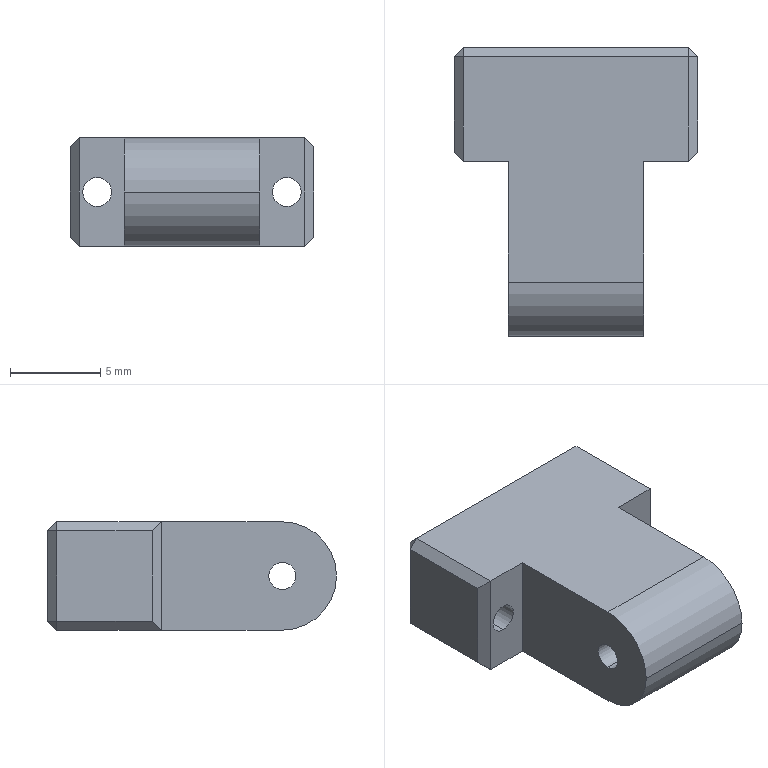Part | SolidWorks | features HoleWzd 2, MirrorPattern 2, Chamfer 1, Extrusion 1, Fillet 1, ICE 1 | 1 solid | 31 faces | box 13.5 x 16 x 6 mm | volume 870.216 mm3 | plane 23 | cylinder 8 | commonest cylinder face diameters 1.6 x4 1.5 x2 6 x2
STEP:
#1=CARTESIAN_POINT('',(9.,-6.3,2.2));
#2=VERTEX_POINT('',#1);
#3=CARTESIAN_POINT('',(9.,-6.3,3.8));
#4=VERTEX_POINT('',#3);
#5=CARTESIAN_POINT('',(9.,-6.3,3.));
#6=DIRECTION('',(0.,1.,0.));
#7=DIRECTION('',(-1.,0.,0.));
#8=AXIS2_PLACEMENT_3D('',#5,#6,#7);
#9=CIRCLE('',#8,0.8);
#10=EDGE_CURVE('',#2,#4,#9,.T.);
#11=ORIENTED_EDGE('',*,*,#10,.F.);
#12=CARTESIAN_POINT('',(9.,0.,2.2));
#13=VERTEX_POINT('',#12);
#14=CARTESIAN_POINT('',(9.,0.,2.2));
#15=DIRECTION('',(0.,1.,0.));
#16=VECTOR('',#15,1000.);
#17=LINE('',#14,#16);
#18=EDGE_CURVE('',#2,#13,#17,.T.);
#19=ORIENTED_EDGE('',*,*,#18,.T.);
#20=CARTESIAN_POINT('',(9.,0.,3.8));
#21=VERTEX_POINT('',#20);
#22=CARTESIAN_POINT('',(9.,0.,3.));
#23=DIRECTION('',(0.,1.,0.));
#24=DIRECTION('',(0.,0.,1.));
#25=AXIS2_PLACEMENT_3D('',#22,#23,#24);
#26=CIRCLE('',#25,0.8);
#27=EDGE_CURVE('',#13,#21,#26,.T.);
#28=ORIENTED_EDGE('',*,*,#27,.T.);
#29=CARTESIAN_POINT('',(9.,0.,3.8));
#30=DIRECTION('',(0.,1.,0.));
#31=VECTOR('',#30,1000.);
#32=LINE('',#29,#31);
#33=EDGE_CURVE('',#4,#21,#32,.T.);
#34=ORIENTED_EDGE('',*,*,#33,.F.);
#35=EDGE_LOOP('',(#11,#19,#28,#34));
#36=FACE_OUTER_BOUND('',#35,.T.);
#37=CARTESIAN_POINT('',(9.,0.,3.));
#38=DIRECTION('',(0.,1.,0.));
#39=DIRECTION('',(0.,0.,1.));
#40=AXIS2_PLACEMENT_3D('',#37,#38,#39);
#41=CYLINDRICAL_SURFACE('',#40,0.8);
#42=ADVANCED_FACE('',(#36),#41,.F.);
#43=CARTESIAN_POINT('',(-1.5,-6.3,3.8));
#44=VERTEX_POINT('',#43);
#45=CARTESIAN_POINT('',(-1.5,-6.3,2.2));
#46=VERTEX_POINT('',#45);
#47=CARTESIAN_POINT('',(-1.5,-6.3,3.));
#48=DIRECTION('',(0.,-1.,0.));
#49=DIRECTION('',(1.,0.,0.));
#50=AXIS2_PLACEMENT_3D('',#47,#48,#49);
#51=CIRCLE('',#50,0.8);
#52=EDGE_CURVE('',#44,#46,#51,.T.);
#53=ORIENTED_EDGE('',*,*,#52,.T.);
#54=CARTESIAN_POINT('',(-1.5,0.,2.2));
#55=VERTEX_POINT('',#54);
#56=CARTESIAN_POINT('',(-1.5,0.,2.2));
#57=DIRECTION('',(0.,1.,0.));
#58=VECTOR('',#57,1000.);
#59=LINE('',#56,#58);
#60=EDGE_CURVE('',#46,#55,#59,.T.);
#61=ORIENTED_EDGE('',*,*,#60,.T.);
#62=CARTESIAN_POINT('',(-1.5,0.,3.8));
#63=VERTEX_POINT('',#62);
#64=CARTESIAN_POINT('',(-1.5,0.,3.));
#65=DIRECTION('',(0.,1.,0.));
#66=DIRECTION('',(0.,0.,1.));
#67=AXIS2_PLACEMENT_3D('',#64,#65,#66);
#68=CIRCLE('',#67,0.8);
#69=EDGE_CURVE('',#55,#63,#68,.T.);
#70=ORIENTED_EDGE('',*,*,#69,.T.);
#71=CARTESIAN_POINT('',(-1.5,0.,3.8));
#72=DIRECTION('',(0.,1.,0.));
#73=VECTOR('',#72,1000.);
#74=LINE('',#71,#73);
#75=EDGE_CURVE('',#44,#63,#74,.T.);
#76=ORIENTED_EDGE('',*,*,#75,.F.);
#77=EDGE_LOOP('',(#53,#61,#70,#76));
#78=FACE_OUTER_BOUND('',#77,.T.);
#79=CARTESIAN_POINT('',(-1.5,0.,3.));
#80=DIRECTION('',(0.,1.,0.));
#81=DIRECTION('',(0.,0.,1.));
#82=AXIS2_PLACEMENT_3D('',#79,#80,#81);
#83=CYLINDRICAL_SURFACE('',#82,0.8);
#84=ADVANCED_FACE('',(#78),#83,.F.);
#85=CARTESIAN_POINT('',(0.,-13.,3.75));
#86=VERTEX_POINT('',#85);
#87=CARTESIAN_POINT('',(0.,-13.,2.25));
#88=VERTEX_POINT('',#87);
#89=CARTESIAN_POINT('',(0.,-13.,3.));
#90=DIRECTION('',(1.,0.,0.));
#91=DIRECTION('',(0.,1.,0.));
#92=AXIS2_PLACEMENT_3D('',#89,#90,#91);
#93=CIRCLE('',#92,0.75);
#94=EDGE_CURVE('',#86,#88,#93,.T.);
#95=ORIENTED_EDGE('',*,*,#94,.F.);
#96=CARTESIAN_POINT('',(7.5,-13.,3.75));
#97=VERTEX_POINT('',#96);
#98=CARTESIAN_POINT('',(7.5,-13.,3.75));
#99=DIRECTION('',(1.,0.,0.));
#100=VECTOR('',#99,1000.);
#101=LINE('',#98,#100);
#102=EDGE_CURVE('',#86,#97,#101,.T.);
#103=ORIENTED_EDGE('',*,*,#102,.T.);
#104=CARTESIAN_POINT('',(7.5,-13.,2.25));
#105=VERTEX_POINT('',#104);
#106=CARTESIAN_POINT('',(7.5,-13.,3.));
#107=DIRECTION('',(1.,0.,0.));
#108=DIRECTION('',(0.,0.,-1.));
#109=AXIS2_PLACEMENT_3D('',#106,#107,#108);
#110=CIRCLE('',#109,0.75);
#111=EDGE_CURVE('',#97,#105,#110,.T.);
#112=ORIENTED_EDGE('',*,*,#111,.T.);
#113=CARTESIAN_POINT('',(7.5,-13.,2.25));
#114=DIRECTION('',(1.,0.,0.));
#115=VECTOR('',#114,1000.);
#116=LINE('',#113,#115);
#117=EDGE_CURVE('',#88,#105,#116,.T.);
#118=ORIENTED_EDGE('',*,*,#117,.F.);
#119=EDGE_LOOP('',(#95,#103,#112,#118));
#120=FACE_OUTER_BOUND('',#119,.T.);
#121=CARTESIAN_POINT('',(7.5,-13.,3.));
#122=DIRECTION('',(1.,0.,0.));
#123=DIRECTION('',(0.,0.,-1.));
#124=AXIS2_PLACEMENT_3D('',#121,#122,#123);
#125=CYLINDRICAL_SURFACE('',#124,0.75);
#126=ADVANCED_FACE('',(#120),#125,.F.);
#127=CARTESIAN_POINT('',(9.,0.,3.));
#128=DIRECTION('',(0.,1.,0.));
#129=DIRECTION('',(0.,0.,1.));
#130=AXIS2_PLACEMENT_3D('',#127,#128,#129);
#131=CIRCLE('',#130,0.8);
#132=EDGE_CURVE('',#21,#13,#131,.T.);
#133=ORIENTED_EDGE('',*,*,#132,.F.);
#134=ORIENTED_EDGE('',*,*,#27,.F.);
#135=EDGE_LOOP('',(#133,#134));
#136=FACE_BOUND('',#135,.T.);
#137=CARTESIAN_POINT('',(-1.5,0.,3.));
#138=DIRECTION('',(0.,1.,0.));
#139=DIRECTION('',(0.,0.,1.));
#140=AXIS2_PLACEMENT_3D('',#137,#138,#139);
#141=CIRCLE('',#140,0.8);
#142=EDGE_CURVE('',#63,#55,#141,.T.);
#143=ORIENTED_EDGE('',*,*,#142,.F.);
#144=ORIENTED_EDGE('',*,*,#69,.F.);
#145=EDGE_LOOP('',(#143,#144));
#146=FACE_BOUND('',#145,.T.);
#147=CARTESIAN_POINT('',(-2.5,0.,5.5));
#148=VERTEX_POINT('',#147);
#149=CARTESIAN_POINT('',(10.,0.,5.5));
#150=VERTEX_POINT('',#149);
#151=CARTESIAN_POINT('',(10.5,0.,5.5));
#152=DIRECTION('',(1.,0.,0.));
#153=VECTOR('',#152,1000.);
#154=LINE('',#151,#153);
#155=EDGE_CURVE('',#148,#150,#154,.T.);
#156=ORIENTED_EDGE('',*,*,#155,.T.);
#157=CARTESIAN_POINT('',(10.,0.,0.5));
#158=VERTEX_POINT('',#157);
#159=CARTESIAN_POINT('',(10.,0.,6.));
#160=DIRECTION('',(0.,0.,-1.));
#161=VECTOR('',#160,1000.);
#162=LINE('',#159,#161);
#163=EDGE_CURVE('',#150,#158,#162,.T.);
#164=ORIENTED_EDGE('',*,*,#163,.T.);
#165=CARTESIAN_POINT('',(-2.5,0.,0.5));
#166=VERTEX_POINT('',#165);
#167=CARTESIAN_POINT('',(0.,0.,0.5));
#168=DIRECTION('',(-1.,0.,0.));
#169=VECTOR('',#168,1000.);
#170=LINE('',#167,#169);
#171=EDGE_CURVE('',#158,#166,#170,.T.);
#172=ORIENTED_EDGE('',*,*,#171,.T.);
#173=CARTESIAN_POINT('',(-2.5,0.,6.));
#174=DIRECTION('',(0.,0.,1.));
#175=VECTOR('',#174,1000.);
#176=LINE('',#173,#175);
#177=EDGE_CURVE('',#166,#148,#176,.T.);
#178=ORIENTED_EDGE('',*,*,#177,.T.);
#179=EDGE_LOOP('',(#156,#164,#172,#178));
#180=FACE_OUTER_BOUND('',#179,.T.);
#181=CARTESIAN_POINT('',(0.,0.,6.));
#182=DIRECTION('',(0.,1.,0.));
#183=DIRECTION('',(0.,0.,1.));
#184=AXIS2_PLACEMENT_3D('',#181,#182,#183);
#185=PLANE('',#184);
#186=ADVANCED_FACE('',(#136,#146,#180),#185,.T.);
#187=CARTESIAN_POINT('',(0.,-13.,3.));
#188=DIRECTION('',(1.,0.,0.));
#189=DIRECTION('',(0.,1.,0.));
#190=AXIS2_PLACEMENT_3D('',#187,#188,#189);
#191=CIRCLE('',#190,0.75);
#192=EDGE_CURVE('',#88,#86,#191,.T.);
#193=ORIENTED_EDGE('',*,*,#192,.T.);
#194=ORIENTED_EDGE('',*,*,#94,.T.);
#195=EDGE_LOOP('',(#193,#194));
#196=FACE_BOUND('',#195,.T.);
#197=CARTESIAN_POINT('',(0.,-6.3,0.));
#198=VERTEX_POINT('',#197);
#199=CARTESIAN_POINT('',(0.,-13.,0.));
#200=VERTEX_POINT('',#199);
#201=CARTESIAN_POINT('',(0.,0.,0.));
#202=DIRECTION('',(0.,-1.,0.));
#203=VECTOR('',#202,1000.);
#204=LINE('',#201,#203);
#205=EDGE_CURVE('',#198,#200,#204,.T.);
#206=ORIENTED_EDGE('',*,*,#205,.T.);
#207=CARTESIAN_POINT('',(0.,-16.,3.));
#208=VERTEX_POINT('',#207);
#209=CARTESIAN_POINT('',(0.,-13.,3.));
#210=DIRECTION('',(-1.,0.,0.));
#211=DIRECTION('',(0.,1.,0.));
#212=AXIS2_PLACEMENT_3D('',#209,#210,#211);
#213=CIRCLE('',#212,3.);
#214=EDGE_CURVE('',#200,#208,#213,.T.);
#215=ORIENTED_EDGE('',*,*,#214,.T.);
#216=CARTESIAN_POINT('',(0.,-13.,6.));
#217=VERTEX_POINT('',#216);
#218=CARTESIAN_POINT('',(0.,-13.,3.));
#219=DIRECTION('',(-1.,0.,0.));
#220=DIRECTION('',(0.,1.,0.));
#221=AXIS2_PLACEMENT_3D('',#218,#219,#220);
#222=CIRCLE('',#221,3.);
#223=EDGE_CURVE('',#208,#217,#222,.T.);
#224=ORIENTED_EDGE('',*,*,#223,.T.);
#225=CARTESIAN_POINT('',(0.,-6.3,6.));
#226=VERTEX_POINT('',#225);
#227=CARTESIAN_POINT('',(0.,0.,6.));
#228=DIRECTION('',(0.,-1.,0.));
#229=VECTOR('',#228,1000.);
#230=LINE('',#227,#229);
#231=EDGE_CURVE('',#226,#217,#230,.T.);
#232=ORIENTED_EDGE('',*,*,#231,.F.);
#233=CARTESIAN_POINT('',(0.,-6.3,6.));
#234=DIRECTION('',(0.,0.,-1.));
#235=VECTOR('',#234,1000.);
#236=LINE('',#233,#235);
#237=EDGE_CURVE('',#226,#198,#236,.T.);
#238=ORIENTED_EDGE('',*,*,#237,.T.);
#239=EDGE_LOOP('',(#206,#215,#224,#232,#238));
#240=FACE_OUTER_BOUND('',#239,.T.);
#241=CARTESIAN_POINT('',(0.,0.,6.));
#242=DIRECTION('',(1.,0.,0.));
#243=DIRECTION('',(0.,1.,0.));
#244=AXIS2_PLACEMENT_3D('',#241,#242,#243);
#245=PLANE('',#244);
#246=ADVANCED_FACE('',(#196,#240),#245,.F.);
#247=CARTESIAN_POINT('',(7.5,-13.,3.));
#248=DIRECTION('',(1.,0.,0.));
#249=DIRECTION('',(0.,0.,-1.));
#250=AXIS2_PLACEMENT_3D('',#247,#248,#249);
#251=CIRCLE('',#250,0.75);
#252=EDGE_CURVE('',#105,#97,#251,.T.);
#253=ORIENTED_EDGE('',*,*,#252,.F.);
#254=ORIENTED_EDGE('',*,*,#111,.F.);
#255=EDGE_LOOP('',(#253,#254));
#256=FACE_BOUND('',#255,.T.);
#257=CARTESIAN_POINT('',(7.5,-13.,6.));
#258=VERTEX_POINT('',#257);
#259=CARTESIAN_POINT('',(7.5,-16.,3.));
#260=VERTEX_POINT('',#259);
#261=CARTESIAN_POINT('',(7.5,-13.,3.));
#262=DIRECTION('',(1.,0.,0.));
#263=DIRECTION('',(0.,1.,0.));
#264=AXIS2_PLACEMENT_3D('',#261,#262,#263);
#265=CIRCLE('',#264,3.);
#266=EDGE_CURVE('',#258,#260,#265,.T.);
#267=ORIENTED_EDGE('',*,*,#266,.T.);
#268=CARTESIAN_POINT('',(7.5,-13.,0.));
#269=VERTEX_POINT('',#268);
#270=CARTESIAN_POINT('',(7.5,-13.,3.));
#271=DIRECTION('',(1.,0.,0.));
#272=DIRECTION('',(0.,1.,0.));
#273=AXIS2_PLACEMENT_3D('',#270,#271,#272);
#274=CIRCLE('',#273,3.);
#275=EDGE_CURVE('',#260,#269,#274,.T.);
#276=ORIENTED_EDGE('',*,*,#275,.T.);
#277=CARTESIAN_POINT('',(7.5,-6.3,0.));
#278=VERTEX_POINT('',#277);
#279=CARTESIAN_POINT('',(7.5,0.,0.));
#280=DIRECTION('',(0.,-1.,0.));
#281=VECTOR('',#280,1000.);
#282=LINE('',#279,#281);
#283=EDGE_CURVE('',#278,#269,#282,.T.);
#284=ORIENTED_EDGE('',*,*,#283,.F.);
#285=CARTESIAN_POINT('',(7.5,-6.3,6.));
#286=VERTEX_POINT('',#285);
#287=CARTESIAN_POINT('',(7.5,-6.3,6.));
#288=DIRECTION('',(0.,0.,-1.));
#289=VECTOR('',#288,1000.);
#290=LINE('',#287,#289);
#291=EDGE_CURVE('',#286,#278,#290,.T.);
#292=ORIENTED_EDGE('',*,*,#291,.F.);
#293=CARTESIAN_POINT('',(7.5,0.,6.));
#294=DIRECTION('',(0.,-1.,0.));
#295=VECTOR('',#294,1000.);
#296=LINE('',#293,#295);
#297=EDGE_CURVE('',#286,#258,#296,.T.);
#298=ORIENTED_EDGE('',*,*,#297,.T.);
#299=EDGE_LOOP('',(#267,#276,#284,#292,#298));
#300=FACE_OUTER_BOUND('',#299,.T.);
#301=CARTESIAN_POINT('',(7.5,0.,6.));
#302=DIRECTION('',(1.,0.,0.));
#303=DIRECTION('',(0.,1.,0.));
#304=AXIS2_PLACEMENT_3D('',#301,#302,#303);
#305=PLANE('',#304);
#306=ADVANCED_FACE('',(#256,#300),#305,.T.);
#307=CARTESIAN_POINT('',(10.,-0.5,6.));
#308=VERTEX_POINT('',#307);
#309=CARTESIAN_POINT('',(-2.5,-0.5,6.));
#310=VERTEX_POINT('',#309);
#311=CARTESIAN_POINT('',(-3.,-0.5,6.));
#312=DIRECTION('',(-1.,0.,0.));
#313=VECTOR('',#312,1000.);
#314=LINE('',#311,#313);
#315=EDGE_CURVE('',#308,#310,#314,.T.);
#316=ORIENTED_EDGE('',*,*,#315,.T.);
#317=CARTESIAN_POINT('',(-2.5,-6.3,6.));
#318=VERTEX_POINT('',#317);
#319=CARTESIAN_POINT('',(-2.5,-6.3,6.));
#320=DIRECTION('',(0.,-1.,0.));
#321=VECTOR('',#320,1000.);
#322=LINE('',#319,#321);
#323=EDGE_CURVE('',#310,#318,#322,.T.);
#324=ORIENTED_EDGE('',*,*,#323,.T.);
#325=CARTESIAN_POINT('',(-3.,-6.3,6.));
#326=DIRECTION('',(1.,0.,0.));
#327=VECTOR('',#326,1000.);
#328=LINE('',#325,#327);
#329=EDGE_CURVE('',#318,#226,#328,.T.);
#330=ORIENTED_EDGE('',*,*,#329,.T.);
#331=ORIENTED_EDGE('',*,*,#231,.T.);
#332=CARTESIAN_POINT('',(0.,-13.,6.));
#333=DIRECTION('',(1.,0.,0.));
#334=VECTOR('',#333,1000.);
#335=LINE('',#332,#334);
#336=EDGE_CURVE('',#217,#258,#335,.T.);
#337=ORIENTED_EDGE('',*,*,#336,.T.);
#338=ORIENTED_EDGE('',*,*,#297,.F.);
#339=CARTESIAN_POINT('',(10.,-6.3,6.));
#340=VERTEX_POINT('',#339);
#341=CARTESIAN_POINT('',(10.5,-6.3,6.));
#342=DIRECTION('',(-1.,0.,0.));
#343=VECTOR('',#342,1000.);
#344=LINE('',#341,#343);
#345=EDGE_CURVE('',#340,#286,#344,.T.);
#346=ORIENTED_EDGE('',*,*,#345,.F.);
#347=CARTESIAN_POINT('',(10.,0.,6.));
#348=DIRECTION('',(0.,1.,0.));
#349=VECTOR('',#348,1000.);
#350=LINE('',#347,#349);
#351=EDGE_CURVE('',#340,#308,#350,.T.);
#352=ORIENTED_EDGE('',*,*,#351,.T.);
#353=EDGE_LOOP('',(#316,#324,#330,#331,#337,#338,#346,#352));
#354=FACE_OUTER_BOUND('',#353,.T.);
#355=CARTESIAN_POINT('',(0.,0.,6.));
#356=DIRECTION('',(0.,0.,-1.));
#357=DIRECTION('',(-1.,0.,0.));
#358=AXIS2_PLACEMENT_3D('',#355,#356,#357);
#359=PLANE('',#358);
#360=ADVANCED_FACE('',(#354),#359,.F.);
#361=CARTESIAN_POINT('',(-2.5,-6.3,0.));
#362=VERTEX_POINT('',#361);
#363=CARTESIAN_POINT('',(-3.,-6.3,0.));
#364=DIRECTION('',(1.,0.,0.));
#365=VECTOR('',#364,1000.);
#366=LINE('',#363,#365);
#367=EDGE_CURVE('',#362,#198,#366,.T.);
#368=ORIENTED_EDGE('',*,*,#367,.F.);
#369=CARTESIAN_POINT('',(-2.5,-0.5,0.));
#370=VERTEX_POINT('',#369);
#371=CARTESIAN_POINT('',(-2.5,0.,0.));
#372=DIRECTION('',(0.,1.,0.));
#373=VECTOR('',#372,1000.);
#374=LINE('',#371,#373);
#375=EDGE_CURVE('',#362,#370,#374,.T.);
#376=ORIENTED_EDGE('',*,*,#375,.T.);
#377=CARTESIAN_POINT('',(10.,-0.5,0.));
#378=VERTEX_POINT('',#377);
#379=CARTESIAN_POINT('',(0.,-0.5,0.));
#380=DIRECTION('',(1.,0.,0.));
#381=VECTOR('',#380,1000.);
#382=LINE('',#379,#381);
#383=EDGE_CURVE('',#370,#378,#382,.T.);
#384=ORIENTED_EDGE('',*,*,#383,.T.);
#385=CARTESIAN_POINT('',(10.,-6.3,0.));
#386=VERTEX_POINT('',#385);
#387=CARTESIAN_POINT('',(10.,0.,0.));
#388=DIRECTION('',(0.,-1.,0.));
#389=VECTOR('',#388,1000.);
#390=LINE('',#387,#389);
#391=EDGE_CURVE('',#378,#386,#390,.T.);
#392=ORIENTED_EDGE('',*,*,#391,.T.);
#393=CARTESIAN_POINT('',(10.5,-6.3,0.));
#394=DIRECTION('',(-1.,0.,0.));
#395=VECTOR('',#394,1000.);
#396=LINE('',#393,#395);
#397=EDGE_CURVE('',#386,#278,#396,.T.);
#398=ORIENTED_EDGE('',*,*,#397,.T.);
#399=ORIENTED_EDGE('',*,*,#283,.T.);
#400=CARTESIAN_POINT('',(0.,-13.,0.));
#401=DIRECTION('',(-1.,0.,0.));
#402=VECTOR('',#401,1000.);
#403=LINE('',#400,#402);
#404=EDGE_CURVE('',#269,#200,#403,.T.);
#405=ORIENTED_EDGE('',*,*,#404,.T.);
#406=ORIENTED_EDGE('',*,*,#205,.F.);
#407=EDGE_LOOP('',(#368,#376,#384,#392,#398,#399,#405,#406));
#408=FACE_OUTER_BOUND('',#407,.T.);
#409=CARTESIAN_POINT('',(0.,0.,0.));
#410=DIRECTION('',(0.,0.,-1.));
#411=DIRECTION('',(-1.,0.,0.));
#412=AXIS2_PLACEMENT_3D('',#409,#410,#411);
#413=PLANE('',#412);
#414=ADVANCED_FACE('',(#408),#413,.T.);
#415=CARTESIAN_POINT('',(9.,-6.3,3.));
#416=DIRECTION('',(0.,1.,0.));
#417=DIRECTION('',(-1.,0.,0.));
#418=AXIS2_PLACEMENT_3D('',#415,#416,#417);
#419=CIRCLE('',#418,0.8);
#420=EDGE_CURVE('',#4,#2,#419,.T.);
#421=ORIENTED_EDGE('',*,*,#420,.T.);
#422=ORIENTED_EDGE('',*,*,#10,.T.);
#423=EDGE_LOOP('',(#421,#422));
#424=FACE_BOUND('',#423,.T.);
#425=ORIENTED_EDGE('',*,*,#397,.F.);
#426=CARTESIAN_POINT('',(10.,-6.3,6.));
#427=DIRECTION('',(0.,0.,1.));
#428=VECTOR('',#427,1000.);
#429=LINE('',#426,#428);
#430=EDGE_CURVE('',#386,#340,#429,.T.);
#431=ORIENTED_EDGE('',*,*,#430,.T.);
#432=ORIENTED_EDGE('',*,*,#345,.T.);
#433=ORIENTED_EDGE('',*,*,#291,.T.);
#434=EDGE_LOOP('',(#425,#431,#432,#433));
#435=FACE_OUTER_BOUND('',#434,.T.);
#436=CARTESIAN_POINT('',(10.5,-6.3,6.));
#437=DIRECTION('',(0.,1.,0.));
#438=DIRECTION('',(-1.,0.,0.));
#439=AXIS2_PLACEMENT_3D('',#436,#437,#438);
#440=PLANE('',#439);
#441=ADVANCED_FACE('',(#424,#435),#440,.F.);
#442=CARTESIAN_POINT('',(10.5,-5.8,5.5));
#443=VERTEX_POINT('',#442);
#444=CARTESIAN_POINT('',(10.5,-5.8,0.5));
#445=VERTEX_POINT('',#444);
#446=CARTESIAN_POINT('',(10.5,-5.8,0.));
#447=DIRECTION('',(0.,0.,-1.));
#448=VECTOR('',#447,1000.);
#449=LINE('',#446,#448);
#450=EDGE_CURVE('',#443,#445,#449,.T.);
#451=ORIENTED_EDGE('',*,*,#450,.T.);
#452=CARTESIAN_POINT('',(10.5,-0.5,0.5));
#453=VERTEX_POINT('',#452);
#454=CARTESIAN_POINT('',(10.5,0.,0.5));
#455=DIRECTION('',(0.,1.,0.));
#456=VECTOR('',#455,1000.);
#457=LINE('',#454,#456);
#458=EDGE_CURVE('',#445,#453,#457,.T.);
#459=ORIENTED_EDGE('',*,*,#458,.T.);
#460=CARTESIAN_POINT('',(10.5,-0.5,5.5));
#461=VERTEX_POINT('',#460);
#462=CARTESIAN_POINT('',(10.5,-0.5,0.));
#463=DIRECTION('',(0.,0.,1.));
#464=VECTOR('',#463,1000.);
#465=LINE('',#462,#464);
#466=EDGE_CURVE('',#453,#461,#465,.T.);
#467=ORIENTED_EDGE('',*,*,#466,.T.);
#468=CARTESIAN_POINT('',(10.5,-6.3,5.5));
#469=DIRECTION('',(0.,-1.,0.));
#470=VECTOR('',#469,1000.);
#471=LINE('',#468,#470);
#472=EDGE_CURVE('',#461,#443,#471,.T.);
#473=ORIENTED_EDGE('',*,*,#472,.T.);
#474=EDGE_LOOP('',(#451,#459,#467,#473));
#475=FACE_OUTER_BOUND('',#474,.T.);
#476=CARTESIAN_POINT('',(10.5,0.,0.));
#477=DIRECTION('',(1.,0.,0.));
#478=DIRECTION('',(0.,1.,0.));
#479=AXIS2_PLACEMENT_3D('',#476,#477,#478);
#480=PLANE('',#479);
#481=ADVANCED_FACE('',(#475),#480,.T.);
#482=ORIENTED_EDGE('',*,*,#52,.F.);
#483=CARTESIAN_POINT('',(-1.5,-6.3,3.));
#484=DIRECTION('',(0.,-1.,0.));
#485=DIRECTION('',(1.,0.,0.));
#486=AXIS2_PLACEMENT_3D('',#483,#484,#485);
#487=CIRCLE('',#486,0.8);
#488=EDGE_CURVE('',#46,#44,#487,.T.);
#489=ORIENTED_EDGE('',*,*,#488,.F.);
#490=EDGE_LOOP('',(#482,#489));
#491=FACE_BOUND('',#490,.T.);
#492=ORIENTED_EDGE('',*,*,#329,.F.);
#493=CARTESIAN_POINT('',(-2.5,-6.3,6.));
#494=DIRECTION('',(0.,0.,-1.));
#495=VECTOR('',#494,1000.);
#496=LINE('',#493,#495);
#497=EDGE_CURVE('',#318,#362,#496,.T.);
#498=ORIENTED_EDGE('',*,*,#497,.T.);
#499=ORIENTED_EDGE('',*,*,#367,.T.);
#500=ORIENTED_EDGE('',*,*,#237,.F.);
#501=EDGE_LOOP('',(#492,#498,#499,#500));
#502=FACE_OUTER_BOUND('',#501,.T.);
#503=CARTESIAN_POINT('',(-3.,-6.3,6.));
#504=DIRECTION('',(0.,-1.,0.));
#505=DIRECTION('',(1.,0.,0.));
#506=AXIS2_PLACEMENT_3D('',#503,#504,#505);
#507=PLANE('',#506);
#508=ADVANCED_FACE('',(#491,#502),#507,.T.);
#509=CARTESIAN_POINT('',(-3.,-0.5,0.5));
#510=VERTEX_POINT('',#509);
#511=CARTESIAN_POINT('',(-3.,-5.8,0.5));
#512=VERTEX_POINT('',#511);
#513=CARTESIAN_POINT('',(-3.,0.,0.5));
#514=DIRECTION('',(0.,-1.,0.));
#515=VECTOR('',#514,1000.);
#516=LINE('',#513,#515);
#517=EDGE_CURVE('',#510,#512,#516,.T.);
#518=ORIENTED_EDGE('',*,*,#517,.T.);
#519=CARTESIAN_POINT('',(-3.,-5.8,5.5));
#520=VERTEX_POINT('',#519);
#521=CARTESIAN_POINT('',(-3.,-5.8,0.));
#522=DIRECTION('',(0.,0.,1.));
#523=VECTOR('',#522,1000.);
#524=LINE('',#521,#523);
#525=EDGE_CURVE('',#512,#520,#524,.T.);
#526=ORIENTED_EDGE('',*,*,#525,.T.);
#527=CARTESIAN_POINT('',(-3.,-0.5,5.5));
#528=VERTEX_POINT('',#527);
#529=CARTESIAN_POINT('',(-3.,0.,5.5));
#530=DIRECTION('',(0.,1.,0.));
#531=VECTOR('',#530,1000.);
#532=LINE('',#529,#531);
#533=EDGE_CURVE('',#520,#528,#532,.T.);
#534=ORIENTED_EDGE('',*,*,#533,.T.);
#535=CARTESIAN_POINT('',(-3.,-0.5,0.));
#536=DIRECTION('',(0.,0.,-1.));
#537=VECTOR('',#536,1000.);
#538=LINE('',#535,#537);
#539=EDGE_CURVE('',#528,#510,#538,.T.);
#540=ORIENTED_EDGE('',*,*,#539,.T.);
#541=EDGE_LOOP('',(#518,#526,#534,#540));
#542=FACE_OUTER_BOUND('',#541,.T.);
#543=CARTESIAN_POINT('',(-3.,0.,0.));
#544=DIRECTION('',(-1.,0.,0.));
#545=DIRECTION('',(0.,1.,0.));
#546=AXIS2_PLACEMENT_3D('',#543,#544,#545);
#547=PLANE('',#546);
#548=ADVANCED_FACE('',(#542),#547,.T.);
#549=ORIENTED_EDGE('',*,*,#102,.F.);
#550=ORIENTED_EDGE('',*,*,#192,.F.);
#551=ORIENTED_EDGE('',*,*,#117,.T.);
#552=ORIENTED_EDGE('',*,*,#252,.T.);
#553=EDGE_LOOP('',(#549,#550,#551,#552));
#554=FACE_OUTER_BOUND('',#553,.T.);
#555=CARTESIAN_POINT('',(7.5,-13.,3.));
#556=DIRECTION('',(1.,0.,0.));
#557=DIRECTION('',(0.,0.,-1.));
#558=AXIS2_PLACEMENT_3D('',#555,#556,#557);
#559=CYLINDRICAL_SURFACE('',#558,0.75);
#560=ADVANCED_FACE('',(#554),#559,.F.);
#561=ORIENTED_EDGE('',*,*,#336,.F.);
#562=ORIENTED_EDGE('',*,*,#223,.F.);
#563=CARTESIAN_POINT('',(0.,-16.,3.));
#564=DIRECTION('',(-1.,0.,0.));
#565=VECTOR('',#564,1000.);
#566=LINE('',#563,#565);
#567=EDGE_CURVE('',#260,#208,#566,.T.);
#568=ORIENTED_EDGE('',*,*,#567,.F.);
#569=ORIENTED_EDGE('',*,*,#266,.F.);
#570=EDGE_LOOP('',(#561,#562,#568,#569));
#571=FACE_OUTER_BOUND('',#570,.T.);
#572=CARTESIAN_POINT('',(0.,-13.,3.));
#573=DIRECTION('',(1.,0.,0.));
#574=DIRECTION('',(0.,0.,-1.));
#575=AXIS2_PLACEMENT_3D('',#572,#573,#574);
#576=CYLINDRICAL_SURFACE('',#575,3.);
#577=ADVANCED_FACE('',(#571),#576,.T.);
#578=ORIENTED_EDGE('',*,*,#214,.F.);
#579=ORIENTED_EDGE('',*,*,#404,.F.);
#580=ORIENTED_EDGE('',*,*,#275,.F.);
#581=ORIENTED_EDGE('',*,*,#567,.T.);
#582=EDGE_LOOP('',(#578,#579,#580,#581));
#583=FACE_OUTER_BOUND('',#582,.T.);
#584=CARTESIAN_POINT('',(0.,-13.,3.));
#585=DIRECTION('',(-1.,0.,0.));
#586=DIRECTION('',(0.,0.,1.));
#587=AXIS2_PLACEMENT_3D('',#584,#585,#586);
#588=CYLINDRICAL_SURFACE('',#587,3.);
#589=ADVANCED_FACE('',(#583),#588,.T.);
#590=CARTESIAN_POINT('',(10.333,-5.967,0.3333));
#591=DIRECTION('',(-0.5774,-0.5774,-0.5774));
#592=VECTOR('',#591,1000.);
#593=LINE('',#590,#592);
#594=EDGE_CURVE('',#445,#386,#593,.T.);
#595=ORIENTED_EDGE('',*,*,#594,.F.);
#596=ORIENTED_EDGE('',*,*,#450,.F.);
#597=CARTESIAN_POINT('',(12.433,-3.867,3.567));
#598=DIRECTION('',(0.5774,0.5774,-0.5774));
#599=VECTOR('',#598,1000.);
#600=LINE('',#597,#599);
#601=EDGE_CURVE('',#340,#443,#600,.T.);
#602=ORIENTED_EDGE('',*,*,#601,.F.);
#603=ORIENTED_EDGE('',*,*,#430,.F.);
#604=EDGE_LOOP('',(#595,#596,#602,#603));
#605=FACE_OUTER_BOUND('',#604,.T.);
#606=CARTESIAN_POINT('',(10.5,-5.8,0.));
#607=DIRECTION('',(0.7071,-0.7071,0.));
#608=DIRECTION('',(0.,0.,1.));
#609=AXIS2_PLACEMENT_3D('',#606,#607,#608);
#610=PLANE('',#609);
#611=ADVANCED_FACE('',(#605),#610,.T.);
#612=ORIENTED_EDGE('',*,*,#601,.T.);
#613=ORIENTED_EDGE('',*,*,#472,.F.);
#614=CARTESIAN_POINT('',(10.,-0.5,6.));
#615=DIRECTION('',(0.7071,0.,-0.7071));
#616=VECTOR('',#615,1000.);
#617=LINE('',#614,#616);
#618=EDGE_CURVE('',#308,#461,#617,.T.);
#619=ORIENTED_EDGE('',*,*,#618,.F.);
#620=ORIENTED_EDGE('',*,*,#351,.F.);
#621=EDGE_LOOP('',(#612,#613,#619,#620));
#622=FACE_OUTER_BOUND('',#621,.T.);
#623=CARTESIAN_POINT('',(10.5,0.,5.5));
#624=DIRECTION('',(0.7071,0.,0.7071));
#625=DIRECTION('',(0.,1.,0.));
#626=AXIS2_PLACEMENT_3D('',#623,#624,#625);
#627=PLANE('',#626);
#628=ADVANCED_FACE('',(#622),#627,.T.);
#629=ORIENTED_EDGE('',*,*,#594,.T.);
#630=ORIENTED_EDGE('',*,*,#391,.F.);
#631=CARTESIAN_POINT('',(10.5,-0.5,0.5));
#632=DIRECTION('',(-0.7071,0.,-0.7071));
#633=VECTOR('',#632,1000.);
#634=LINE('',#631,#633);
#635=EDGE_CURVE('',#453,#378,#634,.T.);
#636=ORIENTED_EDGE('',*,*,#635,.F.);
#637=ORIENTED_EDGE('',*,*,#458,.F.);
#638=EDGE_LOOP('',(#629,#630,#636,#637));
#639=FACE_OUTER_BOUND('',#638,.T.);
#640=CARTESIAN_POINT('',(10.5,0.,0.5));
#641=DIRECTION('',(-0.7071,0.,0.7071));
#642=DIRECTION('',(0.,1.,0.));
#643=AXIS2_PLACEMENT_3D('',#640,#641,#642);
#644=PLANE('',#643);
#645=ADVANCED_FACE('',(#639),#644,.F.);
#646=CARTESIAN_POINT('',(10.25,-0.25,5.5));
#647=DIRECTION('',(-0.7071,0.7071,0.));
#648=VECTOR('',#647,1000.);
#649=LINE('',#646,#648);
#650=EDGE_CURVE('',#461,#150,#649,.T.);
#651=ORIENTED_EDGE('',*,*,#650,.F.);
#652=ORIENTED_EDGE('',*,*,#466,.F.);
#653=CARTESIAN_POINT('',(10.5,-0.5,0.5));
#654=DIRECTION('',(0.7071,-0.7071,0.));
#655=VECTOR('',#654,1000.);
#656=LINE('',#653,#655);
#657=EDGE_CURVE('',#158,#453,#656,.T.);
#658=ORIENTED_EDGE('',*,*,#657,.F.);
#659=ORIENTED_EDGE('',*,*,#163,.F.);
#660=EDGE_LOOP('',(#651,#652,#658,#659));
#661=FACE_OUTER_BOUND('',#660,.T.);
#662=CARTESIAN_POINT('',(10.5,-0.5,0.));
#663=DIRECTION('',(-0.7071,-0.7071,0.));
#664=DIRECTION('',(0.,0.,1.));
#665=AXIS2_PLACEMENT_3D('',#662,#663,#664);
#666=PLANE('',#665);
#667=ADVANCED_FACE('',(#661),#666,.F.);
#668=ORIENTED_EDGE('',*,*,#618,.T.);
#669=ORIENTED_EDGE('',*,*,#650,.T.);
#670=CARTESIAN_POINT('',(10.,-0.5,6.));
#671=DIRECTION('',(0.,0.7071,-0.7071));
#672=VECTOR('',#671,1000.);
#673=LINE('',#670,#672);
#674=EDGE_CURVE('',#308,#150,#673,.T.);
#675=ORIENTED_EDGE('',*,*,#674,.F.);
#676=EDGE_LOOP('',(#668,#669,#675));
#677=FACE_OUTER_BOUND('',#676,.T.);
#678=CARTESIAN_POINT('',(10.,-0.5,6.));
#679=DIRECTION('',(0.5774,0.5774,0.5774));
#680=DIRECTION('',(0.,-0.7071,0.7071));
#681=AXIS2_PLACEMENT_3D('',#678,#679,#680);
#682=PLANE('',#681);
#683=ADVANCED_FACE('',(#677),#682,.T.);
#684=ORIENTED_EDGE('',*,*,#657,.T.);
#685=ORIENTED_EDGE('',*,*,#635,.T.);
#686=CARTESIAN_POINT('',(10.,-0.25,0.25));
#687=DIRECTION('',(0.,-0.7071,-0.7071));
#688=VECTOR('',#687,1000.);
#689=LINE('',#686,#688);
#690=EDGE_CURVE('',#158,#378,#689,.T.);
#691=ORIENTED_EDGE('',*,*,#690,.F.);
#692=EDGE_LOOP('',(#684,#685,#691));
#693=FACE_OUTER_BOUND('',#692,.T.);
#694=CARTESIAN_POINT('',(10.5,-0.5,0.5));
#695=DIRECTION('',(0.5774,0.5774,-0.5774));
#696=DIRECTION('',(-0.7071,0.7071,0.));
#697=AXIS2_PLACEMENT_3D('',#694,#695,#696);
#698=PLANE('',#697);
#699=ADVANCED_FACE('',(#693),#698,.T.);
#700=ORIENTED_EDGE('',*,*,#674,.T.);
#701=ORIENTED_EDGE('',*,*,#155,.F.);
#702=CARTESIAN_POINT('',(-2.5,-0.25,5.75));
#703=DIRECTION('',(0.,0.7071,-0.7071));
#704=VECTOR('',#703,1000.);
#705=LINE('',#702,#704);
#706=EDGE_CURVE('',#310,#148,#705,.T.);
#707=ORIENTED_EDGE('',*,*,#706,.F.);
#708=ORIENTED_EDGE('',*,*,#315,.F.);
#709=EDGE_LOOP('',(#700,#701,#707,#708));
#710=FACE_OUTER_BOUND('',#709,.T.);
#711=CARTESIAN_POINT('',(0.,0.,5.5));
#712=DIRECTION('',(0.,0.7071,0.7071));
#713=DIRECTION('',(-1.,0.,0.));
#714=AXIS2_PLACEMENT_3D('',#711,#712,#713);
#715=PLANE('',#714);
#716=ADVANCED_FACE('',(#710),#715,.T.);
#717=ORIENTED_EDGE('',*,*,#690,.T.);
#718=ORIENTED_EDGE('',*,*,#383,.F.);
#719=CARTESIAN_POINT('',(-2.5,-0.5,0.));
#720=DIRECTION('',(0.,-0.7071,-0.7071));
#721=VECTOR('',#720,1000.);
#722=LINE('',#719,#721);
#723=EDGE_CURVE('',#166,#370,#722,.T.);
#724=ORIENTED_EDGE('',*,*,#723,.F.);
#725=ORIENTED_EDGE('',*,*,#171,.F.);
#726=EDGE_LOOP('',(#717,#718,#724,#725));
#727=FACE_OUTER_BOUND('',#726,.T.);
#728=CARTESIAN_POINT('',(0.,-0.5,0.));
#729=DIRECTION('',(0.,-0.7071,0.7071));
#730=DIRECTION('',(1.,0.,0.));
#731=AXIS2_PLACEMENT_3D('',#728,#729,#730);
#732=PLANE('',#731);
#733=ADVANCED_FACE('',(#727),#732,.F.);
#734=CARTESIAN_POINT('',(-3.,-0.5,5.5));
#735=DIRECTION('',(-0.7071,-0.7071,0.));
#736=VECTOR('',#735,1000.);
#737=LINE('',#734,#736);
#738=EDGE_CURVE('',#148,#528,#737,.T.);
#739=ORIENTED_EDGE('',*,*,#738,.F.);
#740=ORIENTED_EDGE('',*,*,#177,.F.);
#741=CARTESIAN_POINT('',(-2.75,-0.25,0.5));
#742=DIRECTION('',(0.7071,0.7071,0.));
#743=VECTOR('',#742,1000.);
#744=LINE('',#741,#743);
#745=EDGE_CURVE('',#510,#166,#744,.T.);
#746=ORIENTED_EDGE('',*,*,#745,.F.);
#747=ORIENTED_EDGE('',*,*,#539,.F.);
#748=EDGE_LOOP('',(#739,#740,#746,#747));
#749=FACE_OUTER_BOUND('',#748,.T.);
#750=CARTESIAN_POINT('',(-2.5,0.,6.));
#751=DIRECTION('',(0.7071,-0.7071,0.));
#752=DIRECTION('',(0.,0.,1.));
#753=AXIS2_PLACEMENT_3D('',#750,#751,#752);
#754=PLANE('',#753);
#755=ADVANCED_FACE('',(#749),#754,.F.);
#756=ORIENTED_EDGE('',*,*,#706,.T.);
#757=ORIENTED_EDGE('',*,*,#738,.T.);
#758=CARTESIAN_POINT('',(-3.,-0.5,5.5));
#759=DIRECTION('',(-0.7071,0.,-0.7071));
#760=VECTOR('',#759,1000.);
#761=LINE('',#758,#760);
#762=EDGE_CURVE('',#310,#528,#761,.T.);
#763=ORIENTED_EDGE('',*,*,#762,.F.);
#764=EDGE_LOOP('',(#756,#757,#763));
#765=FACE_OUTER_BOUND('',#764,.T.);
#766=CARTESIAN_POINT('',(-3.,-0.5,5.5));
#767=DIRECTION('',(-0.5774,0.5774,0.5774));
#768=DIRECTION('',(-0.7071,-0.7071,0.));
#769=AXIS2_PLACEMENT_3D('',#766,#767,#768);
#770=PLANE('',#769);
#771=ADVANCED_FACE('',(#765),#770,.T.);
#772=ORIENTED_EDGE('',*,*,#745,.T.);
#773=ORIENTED_EDGE('',*,*,#723,.T.);
#774=CARTESIAN_POINT('',(-2.5,-0.5,0.));
#775=DIRECTION('',(0.7071,0.,-0.7071));
#776=VECTOR('',#775,1000.);
#777=LINE('',#774,#776);
#778=EDGE_CURVE('',#510,#370,#777,.T.);
#779=ORIENTED_EDGE('',*,*,#778,.F.);
#780=EDGE_LOOP('',(#772,#773,#779));
#781=FACE_OUTER_BOUND('',#780,.T.);
#782=CARTESIAN_POINT('',(-2.5,-0.5,0.));
#783=DIRECTION('',(-0.5774,0.5774,-0.5774));
#784=DIRECTION('',(-0.7071,-0.7071,0.));
#785=AXIS2_PLACEMENT_3D('',#782,#783,#784);
#786=PLANE('',#785);
#787=ADVANCED_FACE('',(#781),#786,.T.);
#788=ORIENTED_EDGE('',*,*,#762,.T.);
#789=ORIENTED_EDGE('',*,*,#533,.F.);
#790=CARTESIAN_POINT('',(-4.6,-4.2,3.9));
#791=DIRECTION('',(-0.5774,0.5774,-0.5774));
#792=VECTOR('',#791,1000.);
#793=LINE('',#790,#792);
#794=EDGE_CURVE('',#318,#520,#793,.T.);
#795=ORIENTED_EDGE('',*,*,#794,.F.);
#796=ORIENTED_EDGE('',*,*,#323,.F.);
#797=EDGE_LOOP('',(#788,#789,#795,#796));
#798=FACE_OUTER_BOUND('',#797,.T.);
#799=CARTESIAN_POINT('',(-2.5,0.,6.));
#800=DIRECTION('',(-0.7071,0.,0.7071));
#801=DIRECTION('',(0.,1.,0.));
#802=AXIS2_PLACEMENT_3D('',#799,#800,#801);
#803=PLANE('',#802);
#804=ADVANCED_FACE('',(#798),#803,.T.);
#805=ORIENTED_EDGE('',*,*,#778,.T.);
#806=ORIENTED_EDGE('',*,*,#375,.F.);
#807=CARTESIAN_POINT('',(-4.6,-4.2,2.1));
#808=DIRECTION('',(0.5774,-0.5774,-0.5774));
#809=VECTOR('',#808,1000.);
#810=LINE('',#807,#809);
#811=EDGE_CURVE('',#512,#362,#810,.T.);
#812=ORIENTED_EDGE('',*,*,#811,.F.);
#813=ORIENTED_EDGE('',*,*,#517,.F.);
#814=EDGE_LOOP('',(#805,#806,#812,#813));
#815=FACE_OUTER_BOUND('',#814,.T.);
#816=CARTESIAN_POINT('',(-2.5,0.,0.));
#817=DIRECTION('',(0.7071,0.,0.7071));
#818=DIRECTION('',(0.,1.,0.));
#819=AXIS2_PLACEMENT_3D('',#816,#817,#818);
#820=PLANE('',#819);
#821=ADVANCED_FACE('',(#815),#820,.F.);
#822=ORIENTED_EDGE('',*,*,#794,.T.);
#823=ORIENTED_EDGE('',*,*,#525,.F.);
#824=ORIENTED_EDGE('',*,*,#811,.T.);
#825=ORIENTED_EDGE('',*,*,#497,.F.);
#826=EDGE_LOOP('',(#822,#823,#824,#825));
#827=FACE_OUTER_BOUND('',#826,.T.);
#828=CARTESIAN_POINT('',(-2.5,-6.3,6.));
#829=DIRECTION('',(0.7071,0.7071,0.));
#830=DIRECTION('',(0.,0.,-1.));
#831=AXIS2_PLACEMENT_3D('',#828,#829,#830);
#832=PLANE('',#831);
#833=ADVANCED_FACE('',(#827),#832,.F.);
#834=ORIENTED_EDGE('',*,*,#60,.F.);
#835=ORIENTED_EDGE('',*,*,#488,.T.);
#836=ORIENTED_EDGE('',*,*,#75,.T.);
#837=ORIENTED_EDGE('',*,*,#142,.T.);
#838=EDGE_LOOP('',(#834,#835,#836,#837));
#839=FACE_OUTER_BOUND('',#838,.T.);
#840=CARTESIAN_POINT('',(-1.5,0.,3.));
#841=DIRECTION('',(0.,1.,0.));
#842=DIRECTION('',(0.,0.,1.));
#843=AXIS2_PLACEMENT_3D('',#840,#841,#842);
#844=CYLINDRICAL_SURFACE('',#843,0.8);
#845=ADVANCED_FACE('',(#839),#844,.F.);
#846=ORIENTED_EDGE('',*,*,#18,.F.);
#847=ORIENTED_EDGE('',*,*,#420,.F.);
#848=ORIENTED_EDGE('',*,*,#33,.T.);
#849=ORIENTED_EDGE('',*,*,#132,.T.);
#850=EDGE_LOOP('',(#846,#847,#848,#849));
#851=FACE_OUTER_BOUND('',#850,.T.);
#852=CARTESIAN_POINT('',(9.,0.,3.));
#853=DIRECTION('',(0.,1.,0.));
#854=DIRECTION('',(0.,0.,1.));
#855=AXIS2_PLACEMENT_3D('',#852,#853,#854);
#856=CYLINDRICAL_SURFACE('',#855,0.8);
#857=ADVANCED_FACE('',(#851),#856,.F.);
#858=CLOSED_SHELL('',(#42,#84,#126,#186,#246,#306,#360,#414,#441,#481,#508,#548,#560,#577,#589,#611,#628,#645,#667,#683,#699,#716,#733,#755,#771,#787,#804,#821,#833,#845,#857));
#859=MANIFOLD_SOLID_BREP('',#858);
#860=CARTESIAN_POINT('',(0.,0.,0.));
#861=DIRECTION('',(0.,0.,1.));
#862=DIRECTION('',(1.,0.,0.));
#863=AXIS2_PLACEMENT_3D('',#860,#861,#862);
#864=(LENGTH_UNIT()NAMED_UNIT(*)SI_UNIT(.MILLI.,.METRE.));
#865=UNCERTAINTY_MEASURE_WITH_UNIT(LENGTH_MEASURE(0.00001),#864,'','');
#866=(NAMED_UNIT(*)PLANE_ANGLE_UNIT()SI_UNIT($,.RADIAN.));
#867=(NAMED_UNIT(*)SI_UNIT($,.STERADIAN.)SOLID_ANGLE_UNIT());
#868=(GEOMETRIC_REPRESENTATION_CONTEXT(3)GLOBAL_UNCERTAINTY_ASSIGNED_CONTEXT((#865))GLOBAL_UNIT_ASSIGNED_CONTEXT((#864,#866,#867))REPRESENTATION_CONTEXT('',''));
#869=ADVANCED_BREP_SHAPE_REPRESENTATION('',(#859,#863),#868);